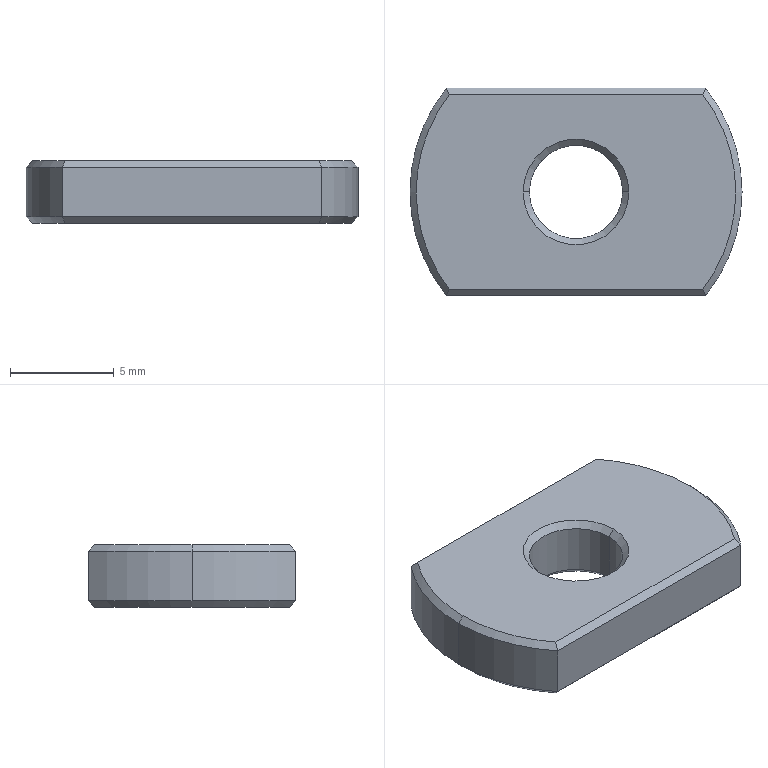Part | SolidWorks | features Chamfer 1, Extrusion 1, ICE 1 | 1 solid | 23 faces | box 16 x 10 x 3 mm | volume 393.425 mm3 | cone 10 | plane 8 | cylinder 5 | commonest cylinder face diameters 16 x3 4.5 x2
STEP:
#1=CARTESIAN_POINT('',(-2.25,0.,1.2));
#2=VERTEX_POINT('',#1);
#3=CARTESIAN_POINT('',(2.25,0.,1.2));
#4=VERTEX_POINT('',#3);
#5=CARTESIAN_POINT('',(0.,0.,1.2));
#6=DIRECTION('',(0.,0.,1.));
#7=DIRECTION('',(1.,0.,0.));
#8=AXIS2_PLACEMENT_3D('',#5,#6,#7);
#9=CIRCLE('',#8,2.25);
#10=EDGE_CURVE('',#2,#4,#9,.T.);
#11=ORIENTED_EDGE('',*,*,#10,.F.);
#12=CARTESIAN_POINT('',(-2.55,0.,1.5));
#13=VERTEX_POINT('',#12);
#14=CARTESIAN_POINT('',(-2.25,0.,1.2));
#15=DIRECTION('',(-0.7071,0.,0.7071));
#16=VECTOR('',#15,1000.);
#17=LINE('',#14,#16);
#18=EDGE_CURVE('',#2,#13,#17,.T.);
#19=ORIENTED_EDGE('',*,*,#18,.T.);
#20=CARTESIAN_POINT('',(2.55,0.,1.5));
#21=VERTEX_POINT('',#20);
#22=CARTESIAN_POINT('',(0.,0.,1.5));
#23=DIRECTION('',(0.,0.,-1.));
#24=DIRECTION('',(1.,0.,0.));
#25=AXIS2_PLACEMENT_3D('',#22,#23,#24);
#26=CIRCLE('',#25,2.55);
#27=EDGE_CURVE('',#21,#13,#26,.T.);
#28=ORIENTED_EDGE('',*,*,#27,.F.);
#29=CARTESIAN_POINT('',(2.25,0.,1.2));
#30=DIRECTION('',(0.7071,0.,0.7071));
#31=VECTOR('',#30,1000.);
#32=LINE('',#29,#31);
#33=EDGE_CURVE('',#4,#21,#32,.T.);
#34=ORIENTED_EDGE('',*,*,#33,.F.);
#35=EDGE_LOOP('',(#11,#19,#28,#34));
#36=FACE_OUTER_BOUND('',#35,.T.);
#37=CARTESIAN_POINT('',(0.,0.,1.2));
#38=DIRECTION('',(0.,0.,1.));
#39=DIRECTION('',(1.,0.,0.));
#40=AXIS2_PLACEMENT_3D('',#37,#38,#39);
#41=CONICAL_SURFACE('',#40,2.25,0.7854);
#42=ADVANCED_FACE('',(#36),#41,.F.);
#43=CARTESIAN_POINT('',(-7.7,0.,1.5));
#44=VERTEX_POINT('',#43);
#45=CARTESIAN_POINT('',(-6.099,-4.7,1.5));
#46=VERTEX_POINT('',#45);
#47=CARTESIAN_POINT('',(0.,0.,1.5));
#48=DIRECTION('',(0.,0.,1.));
#49=DIRECTION('',(1.,0.,0.));
#50=AXIS2_PLACEMENT_3D('',#47,#48,#49);
#51=CIRCLE('',#50,7.7);
#52=EDGE_CURVE('',#44,#46,#51,.T.);
#53=ORIENTED_EDGE('',*,*,#52,.F.);
#54=CARTESIAN_POINT('',(-8.,0.,1.2));
#55=VERTEX_POINT('',#54);
#56=CARTESIAN_POINT('',(-7.7,0.,1.5));
#57=DIRECTION('',(-0.7071,0.,-0.7071));
#58=VECTOR('',#57,1000.);
#59=LINE('',#56,#58);
#60=EDGE_CURVE('',#44,#55,#59,.T.);
#61=ORIENTED_EDGE('',*,*,#60,.T.);
#62=CARTESIAN_POINT('',(-6.245,-5.,1.2));
#63=VERTEX_POINT('',#62);
#64=CARTESIAN_POINT('',(0.,0.,1.2));
#65=DIRECTION('',(0.,0.,-1.));
#66=DIRECTION('',(1.,0.,0.));
#67=AXIS2_PLACEMENT_3D('',#64,#65,#66);
#68=CIRCLE('',#67,8.);
#69=EDGE_CURVE('',#63,#55,#68,.T.);
#70=ORIENTED_EDGE('',*,*,#69,.F.);
#71=CARTESIAN_POINT('',(-6.245,-5.,1.2));
#72=CARTESIAN_POINT('',(-6.197,-4.9,1.3));
#73=CARTESIAN_POINT('',(-6.148,-4.8,1.4));
#74=CARTESIAN_POINT('',(-6.099,-4.7,1.5));
#75=B_SPLINE_CURVE_WITH_KNOTS('',3,(#71,#72,#73,#74),.UNSPECIFIED.,.F.,.F.,(4,4),(0.,0.0004486),.UNSPECIFIED.);
#76=EDGE_CURVE('',#63,#46,#75,.T.);
#77=ORIENTED_EDGE('',*,*,#76,.T.);
#78=EDGE_LOOP('',(#53,#61,#70,#77));
#79=FACE_OUTER_BOUND('',#78,.T.);
#80=CARTESIAN_POINT('',(0.,0.,1.5));
#81=DIRECTION('',(0.,0.,-1.));
#82=DIRECTION('',(-1.,0.,0.));
#83=AXIS2_PLACEMENT_3D('',#80,#81,#82);
#84=CONICAL_SURFACE('',#83,7.7,0.7854);
#85=ADVANCED_FACE('',(#79),#84,.T.);
#86=CARTESIAN_POINT('',(2.25,0.,-1.2));
#87=VERTEX_POINT('',#86);
#88=CARTESIAN_POINT('',(-2.25,0.,-1.2));
#89=VERTEX_POINT('',#88);
#90=CARTESIAN_POINT('',(0.,0.,-1.2));
#91=DIRECTION('',(0.,0.,-1.));
#92=DIRECTION('',(1.,0.,0.));
#93=AXIS2_PLACEMENT_3D('',#90,#91,#92);
#94=CIRCLE('',#93,2.25);
#95=EDGE_CURVE('',#87,#89,#94,.T.);
#96=ORIENTED_EDGE('',*,*,#95,.F.);
#97=CARTESIAN_POINT('',(2.55,0.,-1.5));
#98=VERTEX_POINT('',#97);
#99=CARTESIAN_POINT('',(2.55,0.,-1.5));
#100=DIRECTION('',(0.7071,0.,-0.7071));
#101=VECTOR('',#100,1000.);
#102=LINE('',#99,#101);
#103=EDGE_CURVE('',#87,#98,#102,.T.);
#104=ORIENTED_EDGE('',*,*,#103,.T.);
#105=CARTESIAN_POINT('',(-2.55,0.,-1.5));
#106=VERTEX_POINT('',#105);
#107=CARTESIAN_POINT('',(0.,0.,-1.5));
#108=DIRECTION('',(0.,0.,1.));
#109=DIRECTION('',(1.,0.,0.));
#110=AXIS2_PLACEMENT_3D('',#107,#108,#109);
#111=CIRCLE('',#110,2.55);
#112=EDGE_CURVE('',#106,#98,#111,.T.);
#113=ORIENTED_EDGE('',*,*,#112,.F.);
#114=CARTESIAN_POINT('',(-2.55,0.,-1.5));
#115=DIRECTION('',(-0.7071,0.,-0.7071));
#116=VECTOR('',#115,1000.);
#117=LINE('',#114,#116);
#118=EDGE_CURVE('',#89,#106,#117,.T.);
#119=ORIENTED_EDGE('',*,*,#118,.F.);
#120=EDGE_LOOP('',(#96,#104,#113,#119));
#121=FACE_OUTER_BOUND('',#120,.T.);
#122=CARTESIAN_POINT('',(0.,0.,-1.5));
#123=DIRECTION('',(0.,0.,-1.));
#124=DIRECTION('',(-1.,0.,0.));
#125=AXIS2_PLACEMENT_3D('',#122,#123,#124);
#126=CONICAL_SURFACE('',#125,2.55,0.7854);
#127=ADVANCED_FACE('',(#121),#126,.F.);
#128=CARTESIAN_POINT('',(7.7,0.,-1.5));
#129=VERTEX_POINT('',#128);
#130=CARTESIAN_POINT('',(6.099,-4.7,-1.5));
#131=VERTEX_POINT('',#130);
#132=CARTESIAN_POINT('',(0.,0.,-1.5));
#133=DIRECTION('',(0.,0.,-1.));
#134=DIRECTION('',(1.,0.,0.));
#135=AXIS2_PLACEMENT_3D('',#132,#133,#134);
#136=CIRCLE('',#135,7.7);
#137=EDGE_CURVE('',#129,#131,#136,.T.);
#138=ORIENTED_EDGE('',*,*,#137,.F.);
#139=CARTESIAN_POINT('',(8.,0.,-1.2));
#140=VERTEX_POINT('',#139);
#141=CARTESIAN_POINT('',(8.,0.,-1.2));
#142=DIRECTION('',(0.7071,0.,0.7071));
#143=VECTOR('',#142,1000.);
#144=LINE('',#141,#143);
#145=EDGE_CURVE('',#129,#140,#144,.T.);
#146=ORIENTED_EDGE('',*,*,#145,.T.);
#147=CARTESIAN_POINT('',(6.245,-5.,-1.2));
#148=VERTEX_POINT('',#147);
#149=CARTESIAN_POINT('',(0.,0.,-1.2));
#150=DIRECTION('',(0.,0.,1.));
#151=DIRECTION('',(1.,0.,0.));
#152=AXIS2_PLACEMENT_3D('',#149,#150,#151);
#153=CIRCLE('',#152,8.);
#154=EDGE_CURVE('',#148,#140,#153,.T.);
#155=ORIENTED_EDGE('',*,*,#154,.F.);
#156=CARTESIAN_POINT('',(6.245,-5.,-1.2));
#157=CARTESIAN_POINT('',(6.197,-4.9,-1.3));
#158=CARTESIAN_POINT('',(6.148,-4.8,-1.4));
#159=CARTESIAN_POINT('',(6.099,-4.7,-1.5));
#160=B_SPLINE_CURVE_WITH_KNOTS('',3,(#156,#157,#158,#159),.UNSPECIFIED.,.F.,.F.,(4,4),(0.,0.0004486),.UNSPECIFIED.);
#161=EDGE_CURVE('',#148,#131,#160,.T.);
#162=ORIENTED_EDGE('',*,*,#161,.T.);
#163=EDGE_LOOP('',(#138,#146,#155,#162));
#164=FACE_OUTER_BOUND('',#163,.T.);
#165=CARTESIAN_POINT('',(0.,0.,-1.2));
#166=DIRECTION('',(0.,0.,1.));
#167=DIRECTION('',(1.,0.,0.));
#168=AXIS2_PLACEMENT_3D('',#165,#166,#167);
#169=CONICAL_SURFACE('',#168,8.,0.7854);
#170=ADVANCED_FACE('',(#164),#169,.T.);
#171=ORIENTED_EDGE('',*,*,#10,.T.);
#172=CARTESIAN_POINT('',(2.25,0.,1.5));
#173=DIRECTION('',(0.,0.,-1.));
#174=VECTOR('',#173,1000.);
#175=LINE('',#172,#174);
#176=EDGE_CURVE('',#4,#87,#175,.T.);
#177=ORIENTED_EDGE('',*,*,#176,.T.);
#178=ORIENTED_EDGE('',*,*,#95,.T.);
#179=CARTESIAN_POINT('',(-2.25,0.,1.5));
#180=DIRECTION('',(0.,0.,-1.));
#181=VECTOR('',#180,1000.);
#182=LINE('',#179,#181);
#183=EDGE_CURVE('',#2,#89,#182,.T.);
#184=ORIENTED_EDGE('',*,*,#183,.F.);
#185=EDGE_LOOP('',(#171,#177,#178,#184));
#186=FACE_OUTER_BOUND('',#185,.T.);
#187=CARTESIAN_POINT('',(0.,0.,1.5));
#188=DIRECTION('',(0.,0.,-1.));
#189=DIRECTION('',(-1.,0.,0.));
#190=AXIS2_PLACEMENT_3D('',#187,#188,#189);
#191=CYLINDRICAL_SURFACE('',#190,2.25);
#192=ADVANCED_FACE('',(#186),#191,.F.);
#193=ORIENTED_EDGE('',*,*,#69,.T.);
#194=CARTESIAN_POINT('',(-8.,0.,-1.2));
#195=VERTEX_POINT('',#194);
#196=CARTESIAN_POINT('',(-8.,0.,1.5));
#197=DIRECTION('',(0.,0.,-1.));
#198=VECTOR('',#197,1000.);
#199=LINE('',#196,#198);
#200=EDGE_CURVE('',#55,#195,#199,.T.);
#201=ORIENTED_EDGE('',*,*,#200,.T.);
#202=CARTESIAN_POINT('',(-6.245,-5.,-1.2));
#203=VERTEX_POINT('',#202);
#204=CARTESIAN_POINT('',(0.,0.,-1.2));
#205=DIRECTION('',(0.,0.,1.));
#206=DIRECTION('',(1.,0.,0.));
#207=AXIS2_PLACEMENT_3D('',#204,#205,#206);
#208=CIRCLE('',#207,8.);
#209=EDGE_CURVE('',#195,#203,#208,.T.);
#210=ORIENTED_EDGE('',*,*,#209,.T.);
#211=CARTESIAN_POINT('',(-6.245,-5.,1.5));
#212=DIRECTION('',(0.,0.,-1.));
#213=VECTOR('',#212,1000.);
#214=LINE('',#211,#213);
#215=EDGE_CURVE('',#63,#203,#214,.T.);
#216=ORIENTED_EDGE('',*,*,#215,.F.);
#217=EDGE_LOOP('',(#193,#201,#210,#216));
#218=FACE_OUTER_BOUND('',#217,.T.);
#219=CARTESIAN_POINT('',(0.,0.,1.5));
#220=DIRECTION('',(0.,0.,-1.));
#221=DIRECTION('',(-1.,0.,0.));
#222=AXIS2_PLACEMENT_3D('',#219,#220,#221);
#223=CYLINDRICAL_SURFACE('',#222,8.);
#224=ADVANCED_FACE('',(#218),#223,.T.);
#225=CARTESIAN_POINT('',(6.099,-4.7,1.5));
#226=VERTEX_POINT('',#225);
#227=CARTESIAN_POINT('',(6.099,4.7,1.5));
#228=VERTEX_POINT('',#227);
#229=CARTESIAN_POINT('',(0.,0.,1.5));
#230=DIRECTION('',(0.,0.,1.));
#231=DIRECTION('',(1.,0.,0.));
#232=AXIS2_PLACEMENT_3D('',#229,#230,#231);
#233=CIRCLE('',#232,7.7);
#234=EDGE_CURVE('',#226,#228,#233,.T.);
#235=ORIENTED_EDGE('',*,*,#234,.T.);
#236=CARTESIAN_POINT('',(-6.099,4.7,1.5));
#237=VERTEX_POINT('',#236);
#238=CARTESIAN_POINT('',(0.,4.7,1.5));
#239=DIRECTION('',(-1.,0.,0.));
#240=VECTOR('',#239,1000.);
#241=LINE('',#238,#240);
#242=EDGE_CURVE('',#228,#237,#241,.T.);
#243=ORIENTED_EDGE('',*,*,#242,.T.);
#244=CARTESIAN_POINT('',(0.,0.,1.5));
#245=DIRECTION('',(0.,0.,1.));
#246=DIRECTION('',(1.,0.,0.));
#247=AXIS2_PLACEMENT_3D('',#244,#245,#246);
#248=CIRCLE('',#247,7.7);
#249=EDGE_CURVE('',#237,#44,#248,.T.);
#250=ORIENTED_EDGE('',*,*,#249,.T.);
#251=ORIENTED_EDGE('',*,*,#52,.T.);
#252=CARTESIAN_POINT('',(0.,-4.7,1.5));
#253=DIRECTION('',(1.,0.,0.));
#254=VECTOR('',#253,1000.);
#255=LINE('',#252,#254);
#256=EDGE_CURVE('',#46,#226,#255,.T.);
#257=ORIENTED_EDGE('',*,*,#256,.T.);
#258=EDGE_LOOP('',(#235,#243,#250,#251,#257));
#259=FACE_OUTER_BOUND('',#258,.T.);
#260=ORIENTED_EDGE('',*,*,#27,.T.);
#261=CARTESIAN_POINT('',(0.,0.,1.5));
#262=DIRECTION('',(0.,0.,-1.));
#263=DIRECTION('',(1.,0.,0.));
#264=AXIS2_PLACEMENT_3D('',#261,#262,#263);
#265=CIRCLE('',#264,2.55);
#266=EDGE_CURVE('',#13,#21,#265,.T.);
#267=ORIENTED_EDGE('',*,*,#266,.T.);
#268=EDGE_LOOP('',(#260,#267));
#269=FACE_BOUND('',#268,.T.);
#270=CARTESIAN_POINT('',(0.,0.,1.5));
#271=DIRECTION('',(0.,0.,1.));
#272=DIRECTION('',(1.,0.,0.));
#273=AXIS2_PLACEMENT_3D('',#270,#271,#272);
#274=PLANE('',#273);
#275=ADVANCED_FACE('',(#259,#269),#274,.T.);
#276=CARTESIAN_POINT('',(-6.099,4.7,-1.5));
#277=VERTEX_POINT('',#276);
#278=CARTESIAN_POINT('',(6.099,4.7,-1.5));
#279=VERTEX_POINT('',#278);
#280=CARTESIAN_POINT('',(6.245,4.7,-1.5));
#281=DIRECTION('',(1.,0.,0.));
#282=VECTOR('',#281,1000.);
#283=LINE('',#280,#282);
#284=EDGE_CURVE('',#277,#279,#283,.T.);
#285=ORIENTED_EDGE('',*,*,#284,.T.);
#286=CARTESIAN_POINT('',(0.,0.,-1.5));
#287=DIRECTION('',(0.,0.,-1.));
#288=DIRECTION('',(1.,0.,0.));
#289=AXIS2_PLACEMENT_3D('',#286,#287,#288);
#290=CIRCLE('',#289,7.7);
#291=EDGE_CURVE('',#279,#129,#290,.T.);
#292=ORIENTED_EDGE('',*,*,#291,.T.);
#293=ORIENTED_EDGE('',*,*,#137,.T.);
#294=CARTESIAN_POINT('',(-6.099,-4.7,-1.5));
#295=VERTEX_POINT('',#294);
#296=CARTESIAN_POINT('',(-6.245,-4.7,-1.5));
#297=DIRECTION('',(-1.,0.,0.));
#298=VECTOR('',#297,1000.);
#299=LINE('',#296,#298);
#300=EDGE_CURVE('',#131,#295,#299,.T.);
#301=ORIENTED_EDGE('',*,*,#300,.T.);
#302=CARTESIAN_POINT('',(0.,0.,-1.5));
#303=DIRECTION('',(0.,0.,-1.));
#304=DIRECTION('',(1.,0.,0.));
#305=AXIS2_PLACEMENT_3D('',#302,#303,#304);
#306=CIRCLE('',#305,7.7);
#307=EDGE_CURVE('',#295,#277,#306,.T.);
#308=ORIENTED_EDGE('',*,*,#307,.T.);
#309=EDGE_LOOP('',(#285,#292,#293,#301,#308));
#310=FACE_OUTER_BOUND('',#309,.T.);
#311=ORIENTED_EDGE('',*,*,#112,.T.);
#312=CARTESIAN_POINT('',(0.,0.,-1.5));
#313=DIRECTION('',(0.,0.,1.));
#314=DIRECTION('',(1.,0.,0.));
#315=AXIS2_PLACEMENT_3D('',#312,#313,#314);
#316=CIRCLE('',#315,2.55);
#317=EDGE_CURVE('',#98,#106,#316,.T.);
#318=ORIENTED_EDGE('',*,*,#317,.T.);
#319=EDGE_LOOP('',(#311,#318));
#320=FACE_BOUND('',#319,.T.);
#321=CARTESIAN_POINT('',(0.,0.,-1.5));
#322=DIRECTION('',(0.,0.,1.));
#323=DIRECTION('',(1.,0.,0.));
#324=AXIS2_PLACEMENT_3D('',#321,#322,#323);
#325=PLANE('',#324);
#326=ADVANCED_FACE('',(#310,#320),#325,.F.);
#327=ORIENTED_EDGE('',*,*,#200,.F.);
#328=CARTESIAN_POINT('',(-6.245,5.,1.2));
#329=VERTEX_POINT('',#328);
#330=CARTESIAN_POINT('',(0.,0.,1.2));
#331=DIRECTION('',(0.,0.,-1.));
#332=DIRECTION('',(1.,0.,0.));
#333=AXIS2_PLACEMENT_3D('',#330,#331,#332);
#334=CIRCLE('',#333,8.);
#335=EDGE_CURVE('',#55,#329,#334,.T.);
#336=ORIENTED_EDGE('',*,*,#335,.T.);
#337=CARTESIAN_POINT('',(-6.245,5.,-1.2));
#338=VERTEX_POINT('',#337);
#339=CARTESIAN_POINT('',(-6.245,5.,1.5));
#340=DIRECTION('',(0.,0.,1.));
#341=VECTOR('',#340,1000.);
#342=LINE('',#339,#341);
#343=EDGE_CURVE('',#338,#329,#342,.T.);
#344=ORIENTED_EDGE('',*,*,#343,.F.);
#345=CARTESIAN_POINT('',(0.,0.,-1.2));
#346=DIRECTION('',(0.,0.,1.));
#347=DIRECTION('',(1.,0.,0.));
#348=AXIS2_PLACEMENT_3D('',#345,#346,#347);
#349=CIRCLE('',#348,8.);
#350=EDGE_CURVE('',#338,#195,#349,.T.);
#351=ORIENTED_EDGE('',*,*,#350,.T.);
#352=EDGE_LOOP('',(#327,#336,#344,#351));
#353=FACE_OUTER_BOUND('',#352,.T.);
#354=CARTESIAN_POINT('',(0.,0.,1.5));
#355=DIRECTION('',(0.,0.,-1.));
#356=DIRECTION('',(-1.,0.,0.));
#357=AXIS2_PLACEMENT_3D('',#354,#355,#356);
#358=CYLINDRICAL_SURFACE('',#357,8.);
#359=ADVANCED_FACE('',(#353),#358,.T.);
#360=CARTESIAN_POINT('',(6.245,-5.,1.2));
#361=VERTEX_POINT('',#360);
#362=CARTESIAN_POINT('',(6.245,-5.,1.5));
#363=DIRECTION('',(0.,0.,1.));
#364=VECTOR('',#363,1000.);
#365=LINE('',#362,#364);
#366=EDGE_CURVE('',#148,#361,#365,.T.);
#367=ORIENTED_EDGE('',*,*,#366,.F.);
#368=ORIENTED_EDGE('',*,*,#154,.T.);
#369=CARTESIAN_POINT('',(6.245,5.,-1.2));
#370=VERTEX_POINT('',#369);
#371=CARTESIAN_POINT('',(0.,0.,-1.2));
#372=DIRECTION('',(0.,0.,1.));
#373=DIRECTION('',(1.,0.,0.));
#374=AXIS2_PLACEMENT_3D('',#371,#372,#373);
#375=CIRCLE('',#374,8.);
#376=EDGE_CURVE('',#140,#370,#375,.T.);
#377=ORIENTED_EDGE('',*,*,#376,.T.);
#378=CARTESIAN_POINT('',(6.245,5.,1.2));
#379=VERTEX_POINT('',#378);
#380=CARTESIAN_POINT('',(6.245,5.,1.5));
#381=DIRECTION('',(0.,0.,-1.));
#382=VECTOR('',#381,1000.);
#383=LINE('',#380,#382);
#384=EDGE_CURVE('',#379,#370,#383,.T.);
#385=ORIENTED_EDGE('',*,*,#384,.F.);
#386=CARTESIAN_POINT('',(0.,0.,1.2));
#387=DIRECTION('',(0.,0.,-1.));
#388=DIRECTION('',(1.,0.,0.));
#389=AXIS2_PLACEMENT_3D('',#386,#387,#388);
#390=CIRCLE('',#389,8.);
#391=EDGE_CURVE('',#379,#361,#390,.T.);
#392=ORIENTED_EDGE('',*,*,#391,.T.);
#393=EDGE_LOOP('',(#367,#368,#377,#385,#392));
#394=FACE_OUTER_BOUND('',#393,.T.);
#395=CARTESIAN_POINT('',(0.,0.,1.5));
#396=DIRECTION('',(0.,0.,-1.));
#397=DIRECTION('',(-1.,0.,0.));
#398=AXIS2_PLACEMENT_3D('',#395,#396,#397);
#399=CYLINDRICAL_SURFACE('',#398,8.);
#400=ADVANCED_FACE('',(#394),#399,.T.);
#401=ORIENTED_EDGE('',*,*,#176,.F.);
#402=CARTESIAN_POINT('',(0.,0.,1.2));
#403=DIRECTION('',(0.,0.,1.));
#404=DIRECTION('',(1.,0.,0.));
#405=AXIS2_PLACEMENT_3D('',#402,#403,#404);
#406=CIRCLE('',#405,2.25);
#407=EDGE_CURVE('',#4,#2,#406,.T.);
#408=ORIENTED_EDGE('',*,*,#407,.T.);
#409=ORIENTED_EDGE('',*,*,#183,.T.);
#410=CARTESIAN_POINT('',(0.,0.,-1.2));
#411=DIRECTION('',(0.,0.,-1.));
#412=DIRECTION('',(1.,0.,0.));
#413=AXIS2_PLACEMENT_3D('',#410,#411,#412);
#414=CIRCLE('',#413,2.25);
#415=EDGE_CURVE('',#89,#87,#414,.T.);
#416=ORIENTED_EDGE('',*,*,#415,.T.);
#417=EDGE_LOOP('',(#401,#408,#409,#416));
#418=FACE_OUTER_BOUND('',#417,.T.);
#419=CARTESIAN_POINT('',(0.,0.,1.5));
#420=DIRECTION('',(0.,0.,-1.));
#421=DIRECTION('',(-1.,0.,0.));
#422=AXIS2_PLACEMENT_3D('',#419,#420,#421);
#423=CYLINDRICAL_SURFACE('',#422,2.25);
#424=ADVANCED_FACE('',(#418),#423,.F.);
#425=ORIENTED_EDGE('',*,*,#384,.T.);
#426=CARTESIAN_POINT('',(-6.245,5.,-1.2));
#427=DIRECTION('',(-1.,0.,0.));
#428=VECTOR('',#427,1000.);
#429=LINE('',#426,#428);
#430=EDGE_CURVE('',#370,#338,#429,.T.);
#431=ORIENTED_EDGE('',*,*,#430,.T.);
#432=ORIENTED_EDGE('',*,*,#343,.T.);
#433=CARTESIAN_POINT('',(-10.,5.,1.2));
#434=DIRECTION('',(1.,0.,0.));
#435=VECTOR('',#434,1000.);
#436=LINE('',#433,#435);
#437=EDGE_CURVE('',#329,#379,#436,.T.);
#438=ORIENTED_EDGE('',*,*,#437,.T.);
#439=EDGE_LOOP('',(#425,#431,#432,#438));
#440=FACE_OUTER_BOUND('',#439,.T.);
#441=CARTESIAN_POINT('',(-10.,5.,-1.5));
#442=DIRECTION('',(0.,1.,0.));
#443=DIRECTION('',(0.,0.,1.));
#444=AXIS2_PLACEMENT_3D('',#441,#442,#443);
#445=PLANE('',#444);
#446=ADVANCED_FACE('',(#440),#445,.T.);
#447=ORIENTED_EDGE('',*,*,#215,.T.);
#448=CARTESIAN_POINT('',(6.245,-5.,-1.2));
#449=DIRECTION('',(1.,0.,0.));
#450=VECTOR('',#449,1000.);
#451=LINE('',#448,#450);
#452=EDGE_CURVE('',#203,#148,#451,.T.);
#453=ORIENTED_EDGE('',*,*,#452,.T.);
#454=ORIENTED_EDGE('',*,*,#366,.T.);
#455=CARTESIAN_POINT('',(-10.,-5.,1.2));
#456=DIRECTION('',(-1.,0.,0.));
#457=VECTOR('',#456,1000.);
#458=LINE('',#455,#457);
#459=EDGE_CURVE('',#361,#63,#458,.T.);
#460=ORIENTED_EDGE('',*,*,#459,.T.);
#461=EDGE_LOOP('',(#447,#453,#454,#460));
#462=FACE_OUTER_BOUND('',#461,.T.);
#463=CARTESIAN_POINT('',(-10.,-5.,-1.5));
#464=DIRECTION('',(0.,-1.,0.));
#465=DIRECTION('',(1.,0.,0.));
#466=AXIS2_PLACEMENT_3D('',#463,#464,#465);
#467=PLANE('',#466);
#468=ADVANCED_FACE('',(#462),#467,.T.);
#469=CARTESIAN_POINT('',(-6.099,4.7,-1.5));
#470=CARTESIAN_POINT('',(-6.148,4.8,-1.4));
#471=CARTESIAN_POINT('',(-6.197,4.9,-1.3));
#472=CARTESIAN_POINT('',(-6.245,5.,-1.2));
#473=B_SPLINE_CURVE_WITH_KNOTS('',3,(#469,#470,#471,#472),.UNSPECIFIED.,.F.,.F.,(4,4),(0.,0.0004486),.UNSPECIFIED.);
#474=EDGE_CURVE('',#277,#338,#473,.T.);
#475=ORIENTED_EDGE('',*,*,#474,.F.);
#476=ORIENTED_EDGE('',*,*,#307,.F.);
#477=CARTESIAN_POINT('',(-6.245,-5.,-1.2));
#478=CARTESIAN_POINT('',(-6.197,-4.9,-1.3));
#479=CARTESIAN_POINT('',(-6.148,-4.8,-1.4));
#480=CARTESIAN_POINT('',(-6.099,-4.7,-1.5));
#481=B_SPLINE_CURVE_WITH_KNOTS('',3,(#477,#478,#479,#480),.UNSPECIFIED.,.F.,.F.,(4,4),(0.,0.0004486),.UNSPECIFIED.);
#482=EDGE_CURVE('',#203,#295,#481,.T.);
#483=ORIENTED_EDGE('',*,*,#482,.F.);
#484=ORIENTED_EDGE('',*,*,#209,.F.);
#485=ORIENTED_EDGE('',*,*,#350,.F.);
#486=EDGE_LOOP('',(#475,#476,#483,#484,#485));
#487=FACE_OUTER_BOUND('',#486,.T.);
#488=CARTESIAN_POINT('',(0.,0.,-1.2));
#489=DIRECTION('',(0.,0.,1.));
#490=DIRECTION('',(1.,0.,0.));
#491=AXIS2_PLACEMENT_3D('',#488,#489,#490);
#492=CONICAL_SURFACE('',#491,8.,0.7854);
#493=ADVANCED_FACE('',(#487),#492,.T.);
#494=ORIENTED_EDGE('',*,*,#482,.T.);
#495=ORIENTED_EDGE('',*,*,#300,.F.);
#496=ORIENTED_EDGE('',*,*,#161,.F.);
#497=ORIENTED_EDGE('',*,*,#452,.F.);
#498=EDGE_LOOP('',(#494,#495,#496,#497));
#499=FACE_OUTER_BOUND('',#498,.T.);
#500=CARTESIAN_POINT('',(-10.,-5.,-1.2));
#501=DIRECTION('',(0.,-0.7071,-0.7071));
#502=DIRECTION('',(-1.,0.,0.));
#503=AXIS2_PLACEMENT_3D('',#500,#501,#502);
#504=PLANE('',#503);
#505=ADVANCED_FACE('',(#499),#504,.T.);
#506=ORIENTED_EDGE('',*,*,#474,.T.);
#507=ORIENTED_EDGE('',*,*,#430,.F.);
#508=CARTESIAN_POINT('',(6.099,4.7,-1.5));
#509=CARTESIAN_POINT('',(6.148,4.8,-1.4));
#510=CARTESIAN_POINT('',(6.197,4.9,-1.3));
#511=CARTESIAN_POINT('',(6.245,5.,-1.2));
#512=B_SPLINE_CURVE_WITH_KNOTS('',3,(#508,#509,#510,#511),.UNSPECIFIED.,.F.,.F.,(4,4),(0.,0.0004486),.UNSPECIFIED.);
#513=EDGE_CURVE('',#279,#370,#512,.T.);
#514=ORIENTED_EDGE('',*,*,#513,.F.);
#515=ORIENTED_EDGE('',*,*,#284,.F.);
#516=EDGE_LOOP('',(#506,#507,#514,#515));
#517=FACE_OUTER_BOUND('',#516,.T.);
#518=CARTESIAN_POINT('',(-10.,5.,-1.2));
#519=DIRECTION('',(0.,0.7071,-0.7071));
#520=DIRECTION('',(1.,0.,0.));
#521=AXIS2_PLACEMENT_3D('',#518,#519,#520);
#522=PLANE('',#521);
#523=ADVANCED_FACE('',(#517),#522,.T.);
#524=ORIENTED_EDGE('',*,*,#145,.F.);
#525=ORIENTED_EDGE('',*,*,#291,.F.);
#526=ORIENTED_EDGE('',*,*,#513,.T.);
#527=ORIENTED_EDGE('',*,*,#376,.F.);
#528=EDGE_LOOP('',(#524,#525,#526,#527));
#529=FACE_OUTER_BOUND('',#528,.T.);
#530=CARTESIAN_POINT('',(0.,0.,-1.2));
#531=DIRECTION('',(0.,0.,1.));
#532=DIRECTION('',(1.,0.,0.));
#533=AXIS2_PLACEMENT_3D('',#530,#531,#532);
#534=CONICAL_SURFACE('',#533,8.,0.7854);
#535=ADVANCED_FACE('',(#529),#534,.T.);
#536=ORIENTED_EDGE('',*,*,#103,.F.);
#537=ORIENTED_EDGE('',*,*,#415,.F.);
#538=ORIENTED_EDGE('',*,*,#118,.T.);
#539=ORIENTED_EDGE('',*,*,#317,.F.);
#540=EDGE_LOOP('',(#536,#537,#538,#539));
#541=FACE_OUTER_BOUND('',#540,.T.);
#542=CARTESIAN_POINT('',(0.,0.,-1.5));
#543=DIRECTION('',(0.,0.,-1.));
#544=DIRECTION('',(-1.,0.,0.));
#545=AXIS2_PLACEMENT_3D('',#542,#543,#544);
#546=CONICAL_SURFACE('',#545,2.55,0.7854);
#547=ADVANCED_FACE('',(#541),#546,.F.);
#548=ORIENTED_EDGE('',*,*,#76,.F.);
#549=ORIENTED_EDGE('',*,*,#459,.F.);
#550=CARTESIAN_POINT('',(6.099,-4.7,1.5));
#551=CARTESIAN_POINT('',(6.148,-4.8,1.4));
#552=CARTESIAN_POINT('',(6.197,-4.9,1.3));
#553=CARTESIAN_POINT('',(6.245,-5.,1.2));
#554=B_SPLINE_CURVE_WITH_KNOTS('',3,(#550,#551,#552,#553),.UNSPECIFIED.,.F.,.F.,(4,4),(0.,0.0004486),.UNSPECIFIED.);
#555=EDGE_CURVE('',#226,#361,#554,.T.);
#556=ORIENTED_EDGE('',*,*,#555,.F.);
#557=ORIENTED_EDGE('',*,*,#256,.F.);
#558=EDGE_LOOP('',(#548,#549,#556,#557));
#559=FACE_OUTER_BOUND('',#558,.T.);
#560=CARTESIAN_POINT('',(0.,-4.7,1.5));
#561=DIRECTION('',(0.,0.7071,-0.7071));
#562=DIRECTION('',(1.,0.,0.));
#563=AXIS2_PLACEMENT_3D('',#560,#561,#562);
#564=PLANE('',#563);
#565=ADVANCED_FACE('',(#559),#564,.F.);
#566=ORIENTED_EDGE('',*,*,#555,.T.);
#567=ORIENTED_EDGE('',*,*,#391,.F.);
#568=CARTESIAN_POINT('',(6.099,4.7,1.5));
#569=CARTESIAN_POINT('',(6.148,4.8,1.4));
#570=CARTESIAN_POINT('',(6.197,4.9,1.3));
#571=CARTESIAN_POINT('',(6.245,5.,1.2));
#572=B_SPLINE_CURVE_WITH_KNOTS('',3,(#568,#569,#570,#571),.UNSPECIFIED.,.F.,.F.,(4,4),(0.,0.0004486),.UNSPECIFIED.);
#573=EDGE_CURVE('',#228,#379,#572,.T.);
#574=ORIENTED_EDGE('',*,*,#573,.F.);
#575=ORIENTED_EDGE('',*,*,#234,.F.);
#576=EDGE_LOOP('',(#566,#567,#574,#575));
#577=FACE_OUTER_BOUND('',#576,.T.);
#578=CARTESIAN_POINT('',(0.,0.,1.5));
#579=DIRECTION('',(0.,0.,-1.));
#580=DIRECTION('',(-1.,0.,0.));
#581=AXIS2_PLACEMENT_3D('',#578,#579,#580);
#582=CONICAL_SURFACE('',#581,7.7,0.7854);
#583=ADVANCED_FACE('',(#577),#582,.T.);
#584=ORIENTED_EDGE('',*,*,#60,.F.);
#585=ORIENTED_EDGE('',*,*,#249,.F.);
#586=CARTESIAN_POINT('',(-6.245,5.,1.2));
#587=CARTESIAN_POINT('',(-6.197,4.9,1.3));
#588=CARTESIAN_POINT('',(-6.148,4.8,1.4));
#589=CARTESIAN_POINT('',(-6.099,4.7,1.5));
#590=B_SPLINE_CURVE_WITH_KNOTS('',3,(#586,#587,#588,#589),.UNSPECIFIED.,.F.,.F.,(4,4),(0.,0.0004486),.UNSPECIFIED.);
#591=EDGE_CURVE('',#329,#237,#590,.T.);
#592=ORIENTED_EDGE('',*,*,#591,.F.);
#593=ORIENTED_EDGE('',*,*,#335,.F.);
#594=EDGE_LOOP('',(#584,#585,#592,#593));
#595=FACE_OUTER_BOUND('',#594,.T.);
#596=CARTESIAN_POINT('',(0.,0.,1.5));
#597=DIRECTION('',(0.,0.,-1.));
#598=DIRECTION('',(-1.,0.,0.));
#599=AXIS2_PLACEMENT_3D('',#596,#597,#598);
#600=CONICAL_SURFACE('',#599,7.7,0.7854);
#601=ADVANCED_FACE('',(#595),#600,.T.);
#602=ORIENTED_EDGE('',*,*,#573,.T.);
#603=ORIENTED_EDGE('',*,*,#437,.F.);
#604=ORIENTED_EDGE('',*,*,#591,.T.);
#605=ORIENTED_EDGE('',*,*,#242,.F.);
#606=EDGE_LOOP('',(#602,#603,#604,#605));
#607=FACE_OUTER_BOUND('',#606,.T.);
#608=CARTESIAN_POINT('',(0.,4.7,1.5));
#609=DIRECTION('',(0.,-0.7071,-0.7071));
#610=DIRECTION('',(-1.,0.,0.));
#611=AXIS2_PLACEMENT_3D('',#608,#609,#610);
#612=PLANE('',#611);
#613=ADVANCED_FACE('',(#607),#612,.F.);
#614=ORIENTED_EDGE('',*,*,#18,.F.);
#615=ORIENTED_EDGE('',*,*,#407,.F.);
#616=ORIENTED_EDGE('',*,*,#33,.T.);
#617=ORIENTED_EDGE('',*,*,#266,.F.);
#618=EDGE_LOOP('',(#614,#615,#616,#617));
#619=FACE_OUTER_BOUND('',#618,.T.);
#620=CARTESIAN_POINT('',(0.,0.,1.2));
#621=DIRECTION('',(0.,0.,1.));
#622=DIRECTION('',(1.,0.,0.));
#623=AXIS2_PLACEMENT_3D('',#620,#621,#622);
#624=CONICAL_SURFACE('',#623,2.25,0.7854);
#625=ADVANCED_FACE('',(#619),#624,.F.);
#626=CLOSED_SHELL('',(#42,#85,#127,#170,#192,#224,#275,#326,#359,#400,#424,#446,#468,#493,#505,#523,#535,#547,#565,#583,#601,#613,#625));
#627=MANIFOLD_SOLID_BREP('',#626);
#628=CARTESIAN_POINT('',(0.,0.,0.));
#629=DIRECTION('',(0.,0.,1.));
#630=DIRECTION('',(1.,0.,0.));
#631=AXIS2_PLACEMENT_3D('',#628,#629,#630);
#632=(LENGTH_UNIT()NAMED_UNIT(*)SI_UNIT(.MILLI.,.METRE.));
#633=UNCERTAINTY_MEASURE_WITH_UNIT(LENGTH_MEASURE(0.00001),#632,'','');
#634=(NAMED_UNIT(*)PLANE_ANGLE_UNIT()SI_UNIT($,.RADIAN.));
#635=(NAMED_UNIT(*)SI_UNIT($,.STERADIAN.)SOLID_ANGLE_UNIT());
#636=(GEOMETRIC_REPRESENTATION_CONTEXT(3)GLOBAL_UNCERTAINTY_ASSIGNED_CONTEXT((#633))GLOBAL_UNIT_ASSIGNED_CONTEXT((#632,#634,#635))REPRESENTATION_CONTEXT('',''));
#637=ADVANCED_BREP_SHAPE_REPRESENTATION('',(#627,#631),#636);